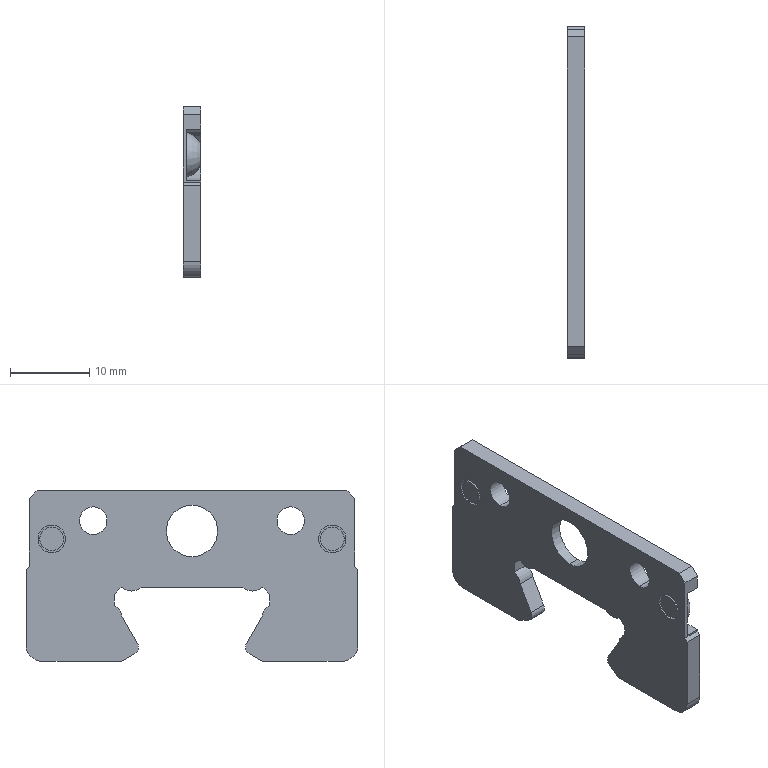Part | NX | 1 solid | 83 faces | box 2.25 x 42 x 21.6 mm | volume 1439 mm3 | plane 49 | cylinder 26 | cone 4 | torus 4 | commonest cylinder face diameters 3.5 x8 3 x4 3.6 x4 6.5 x4 2 x2 4 x2